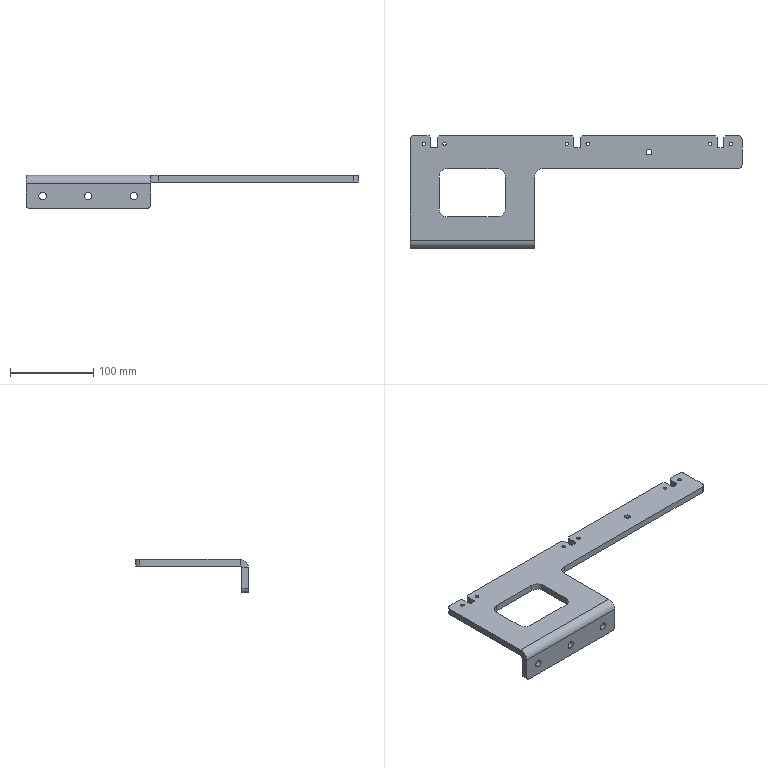Part | SolidWorks | features MirrorStock 1 | 1 solid | 74 faces | box 400 x 136 x 40 mm | volume 236544 mm3 | cylinder 38 | plane 36 | commonest cylinder face diameters 4.2 x12 4 x7 9 x6 20 x6 10 x5 6.8 x2